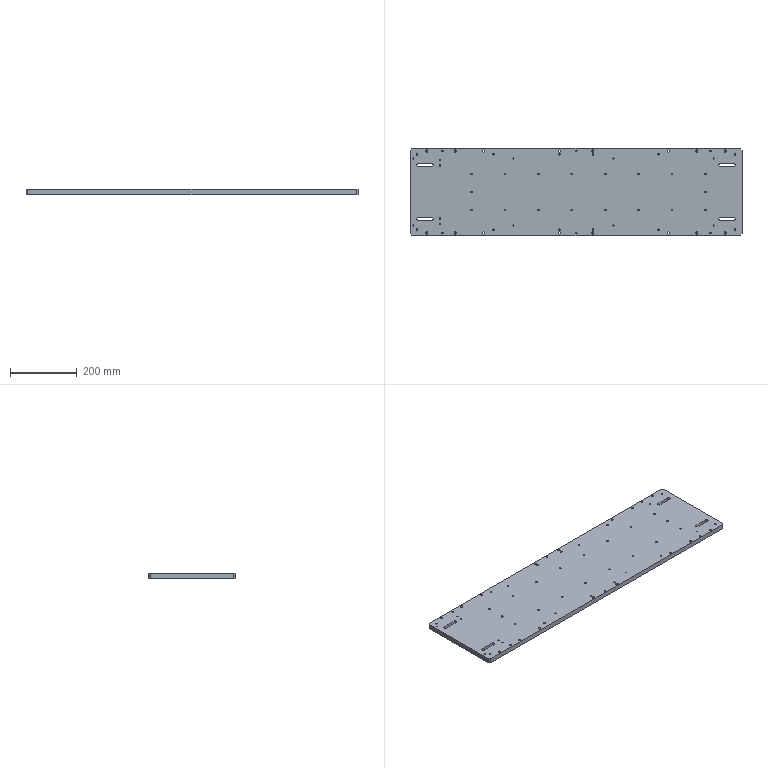Part | 1 solid | 90 faces | box 995 x 261 x 15 mm | volume 3847092 mm3 | cylinder 72 | plane 18 | commonest cylinder face diameters 5 x18 5.1 x16 6.8 x16 3.3 x8 9 x8 4.2 x4